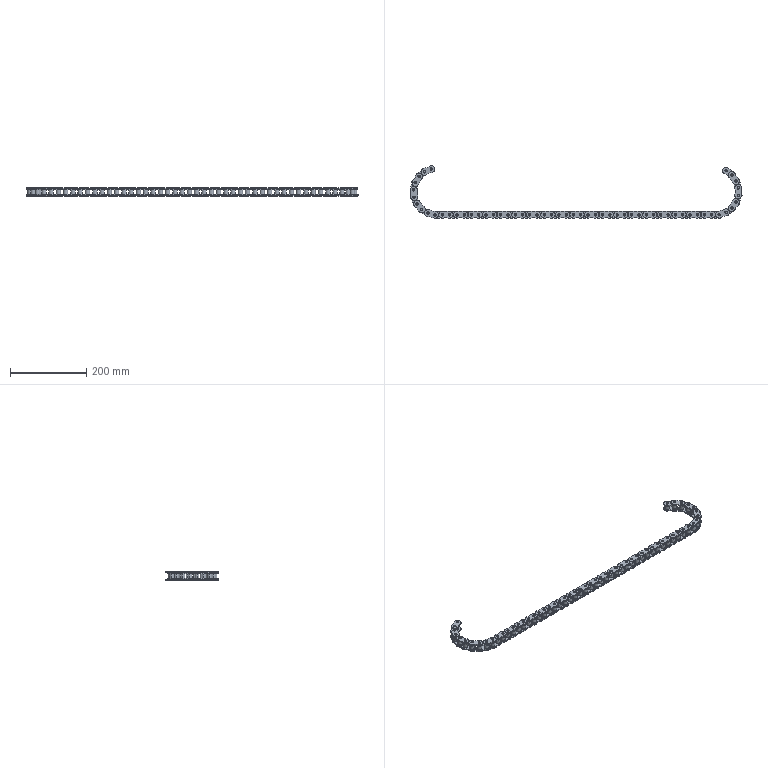Part | SolidWorks | features BaseBody 84 | 84 solids | 1696 faces | box 868.422 x 138.131 x 25.52 mm | volume 250514 mm3 | cylinder 1136 | plane 336 | cone 224 | commonest cylinder face diameters 5.96 x448 18.08 x348 83.184 x228 11.91 x112